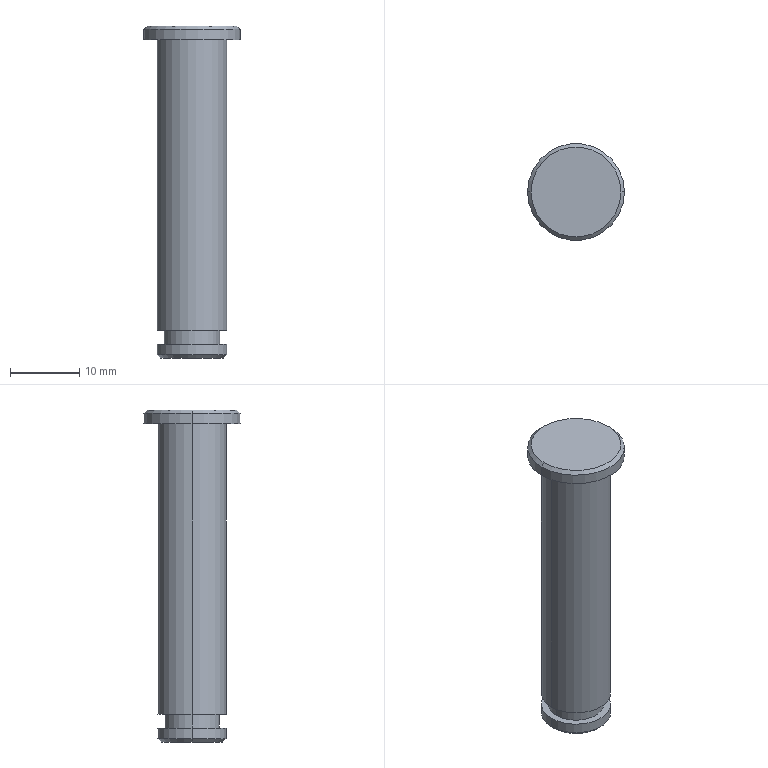Part | SolidWorks | features Chamfer 1, CutThin 1, Extrusion 1, ICE 1 | 1 solid | 17 faces | box 14 x 14 x 48 mm | volume 3855 mm3 | cylinder 8 | plane 5 | cone 4 | commonest cylinder face diameters 10 x4 8 x2 14 x2
STEP:
#1=CARTESIAN_POINT('',(-5.,0.,2.));
#2=VERTEX_POINT('',#1);
#3=CARTESIAN_POINT('',(5.,0.,2.));
#4=VERTEX_POINT('',#3);
#5=CARTESIAN_POINT('',(0.,0.,2.));
#6=DIRECTION('',(0.,0.,-1.));
#7=DIRECTION('',(-1.,0.,0.));
#8=AXIS2_PLACEMENT_3D('',#5,#6,#7);
#9=CIRCLE('',#8,5.);
#10=EDGE_CURVE('',#2,#4,#9,.T.);
#11=ORIENTED_EDGE('',*,*,#10,.T.);
#12=CARTESIAN_POINT('',(5.,0.,0.5));
#13=VERTEX_POINT('',#12);
#14=CARTESIAN_POINT('',(5.,0.,46.));
#15=DIRECTION('',(0.,0.,-1.));
#16=VECTOR('',#15,1000.);
#17=LINE('',#14,#16);
#18=EDGE_CURVE('',#4,#13,#17,.T.);
#19=ORIENTED_EDGE('',*,*,#18,.T.);
#20=CARTESIAN_POINT('',(-5.,0.,0.5));
#21=VERTEX_POINT('',#20);
#22=CARTESIAN_POINT('',(0.,0.,0.5));
#23=DIRECTION('',(0.,0.,1.));
#24=DIRECTION('',(1.,0.,0.));
#25=AXIS2_PLACEMENT_3D('',#22,#23,#24);
#26=CIRCLE('',#25,5.);
#27=EDGE_CURVE('',#13,#21,#26,.T.);
#28=ORIENTED_EDGE('',*,*,#27,.T.);
#29=CARTESIAN_POINT('',(-5.,0.,46.));
#30=DIRECTION('',(0.,0.,-1.));
#31=VECTOR('',#30,1000.);
#32=LINE('',#29,#31);
#33=EDGE_CURVE('',#2,#21,#32,.T.);
#34=ORIENTED_EDGE('',*,*,#33,.F.);
#35=EDGE_LOOP('',(#11,#19,#28,#34));
#36=FACE_OUTER_BOUND('',#35,.T.);
#37=CARTESIAN_POINT('',(0.,0.,46.));
#38=DIRECTION('',(0.,0.,-1.));
#39=DIRECTION('',(-1.,0.,0.));
#40=AXIS2_PLACEMENT_3D('',#37,#38,#39);
#41=CYLINDRICAL_SURFACE('',#40,5.);
#42=ADVANCED_FACE('',(#36),#41,.T.);
#43=CARTESIAN_POINT('',(-4.5,0.,0.));
#44=VERTEX_POINT('',#43);
#45=CARTESIAN_POINT('',(4.5,0.,0.));
#46=VERTEX_POINT('',#45);
#47=CARTESIAN_POINT('',(0.,0.,0.));
#48=DIRECTION('',(0.,0.,-1.));
#49=DIRECTION('',(1.,0.,0.));
#50=AXIS2_PLACEMENT_3D('',#47,#48,#49);
#51=CIRCLE('',#50,4.5);
#52=EDGE_CURVE('',#44,#46,#51,.T.);
#53=ORIENTED_EDGE('',*,*,#52,.F.);
#54=CARTESIAN_POINT('',(-5.,0.,0.5));
#55=DIRECTION('',(-0.7071,0.,0.7071));
#56=VECTOR('',#55,1000.);
#57=LINE('',#54,#56);
#58=EDGE_CURVE('',#44,#21,#57,.T.);
#59=ORIENTED_EDGE('',*,*,#58,.T.);
#60=ORIENTED_EDGE('',*,*,#27,.F.);
#61=CARTESIAN_POINT('',(5.,0.,0.5));
#62=DIRECTION('',(0.7071,0.,0.7071));
#63=VECTOR('',#62,1000.);
#64=LINE('',#61,#63);
#65=EDGE_CURVE('',#46,#13,#64,.T.);
#66=ORIENTED_EDGE('',*,*,#65,.F.);
#67=EDGE_LOOP('',(#53,#59,#60,#66));
#68=FACE_OUTER_BOUND('',#67,.T.);
#69=CARTESIAN_POINT('',(0.,0.,0.5));
#70=DIRECTION('',(0.,0.,1.));
#71=DIRECTION('',(1.,0.,0.));
#72=AXIS2_PLACEMENT_3D('',#69,#70,#71);
#73=CONICAL_SURFACE('',#72,5.,0.7854);
#74=ADVANCED_FACE('',(#68),#73,.T.);
#75=CARTESIAN_POINT('',(-4.,0.,4.));
#76=VERTEX_POINT('',#75);
#77=CARTESIAN_POINT('',(4.,0.,4.));
#78=VERTEX_POINT('',#77);
#79=CARTESIAN_POINT('',(0.,0.,4.));
#80=DIRECTION('',(0.,0.,-1.));
#81=DIRECTION('',(-1.,0.,0.));
#82=AXIS2_PLACEMENT_3D('',#79,#80,#81);
#83=CIRCLE('',#82,4.);
#84=EDGE_CURVE('',#76,#78,#83,.T.);
#85=ORIENTED_EDGE('',*,*,#84,.T.);
#86=CARTESIAN_POINT('',(4.,0.,2.));
#87=VERTEX_POINT('',#86);
#88=CARTESIAN_POINT('',(4.,0.,4.));
#89=DIRECTION('',(0.,0.,-1.));
#90=VECTOR('',#89,1000.);
#91=LINE('',#88,#90);
#92=EDGE_CURVE('',#78,#87,#91,.T.);
#93=ORIENTED_EDGE('',*,*,#92,.T.);
#94=CARTESIAN_POINT('',(-4.,0.,2.));
#95=VERTEX_POINT('',#94);
#96=CARTESIAN_POINT('',(0.,0.,2.));
#97=DIRECTION('',(0.,0.,-1.));
#98=DIRECTION('',(-1.,0.,0.));
#99=AXIS2_PLACEMENT_3D('',#96,#97,#98);
#100=CIRCLE('',#99,4.);
#101=EDGE_CURVE('',#95,#87,#100,.T.);
#102=ORIENTED_EDGE('',*,*,#101,.F.);
#103=CARTESIAN_POINT('',(-4.,0.,4.));
#104=DIRECTION('',(0.,0.,-1.));
#105=VECTOR('',#104,1000.);
#106=LINE('',#103,#105);
#107=EDGE_CURVE('',#76,#95,#106,.T.);
#108=ORIENTED_EDGE('',*,*,#107,.F.);
#109=EDGE_LOOP('',(#85,#93,#102,#108));
#110=FACE_OUTER_BOUND('',#109,.T.);
#111=CARTESIAN_POINT('',(0.,0.,4.));
#112=DIRECTION('',(0.,0.,-1.));
#113=DIRECTION('',(-1.,0.,0.));
#114=AXIS2_PLACEMENT_3D('',#111,#112,#113);
#115=CYLINDRICAL_SURFACE('',#114,4.);
#116=ADVANCED_FACE('',(#110),#115,.T.);
#117=CARTESIAN_POINT('',(6.5,0.,48.));
#118=VERTEX_POINT('',#117);
#119=CARTESIAN_POINT('',(-6.5,0.,48.));
#120=VERTEX_POINT('',#119);
#121=CARTESIAN_POINT('',(0.,0.,48.));
#122=DIRECTION('',(0.,0.,1.));
#123=DIRECTION('',(1.,0.,0.));
#124=AXIS2_PLACEMENT_3D('',#121,#122,#123);
#125=CIRCLE('',#124,6.5);
#126=EDGE_CURVE('',#118,#120,#125,.T.);
#127=ORIENTED_EDGE('',*,*,#126,.F.);
#128=CARTESIAN_POINT('',(7.,0.,47.5));
#129=VERTEX_POINT('',#128);
#130=CARTESIAN_POINT('',(6.5,0.,48.));
#131=DIRECTION('',(0.7071,0.,-0.7071));
#132=VECTOR('',#131,1000.);
#133=LINE('',#130,#132);
#134=EDGE_CURVE('',#118,#129,#133,.T.);
#135=ORIENTED_EDGE('',*,*,#134,.T.);
#136=CARTESIAN_POINT('',(-7.,0.,47.5));
#137=VERTEX_POINT('',#136);
#138=CARTESIAN_POINT('',(0.,0.,47.5));
#139=DIRECTION('',(0.,0.,-1.));
#140=DIRECTION('',(1.,0.,0.));
#141=AXIS2_PLACEMENT_3D('',#138,#139,#140);
#142=CIRCLE('',#141,7.);
#143=EDGE_CURVE('',#137,#129,#142,.T.);
#144=ORIENTED_EDGE('',*,*,#143,.F.);
#145=CARTESIAN_POINT('',(-6.5,0.,48.));
#146=DIRECTION('',(-0.7071,0.,-0.7071));
#147=VECTOR('',#146,1000.);
#148=LINE('',#145,#147);
#149=EDGE_CURVE('',#120,#137,#148,.T.);
#150=ORIENTED_EDGE('',*,*,#149,.F.);
#151=EDGE_LOOP('',(#127,#135,#144,#150));
#152=FACE_OUTER_BOUND('',#151,.T.);
#153=CARTESIAN_POINT('',(0.,0.,48.));
#154=DIRECTION('',(0.,0.,-1.));
#155=DIRECTION('',(-1.,0.,0.));
#156=AXIS2_PLACEMENT_3D('',#153,#154,#155);
#157=CONICAL_SURFACE('',#156,6.5,0.7854);
#158=ADVANCED_FACE('',(#152),#157,.T.);
#159=ORIENTED_EDGE('',*,*,#143,.T.);
#160=CARTESIAN_POINT('',(7.,0.,46.));
#161=VERTEX_POINT('',#160);
#162=CARTESIAN_POINT('',(7.,0.,48.));
#163=DIRECTION('',(0.,0.,-1.));
#164=VECTOR('',#163,1000.);
#165=LINE('',#162,#164);
#166=EDGE_CURVE('',#129,#161,#165,.T.);
#167=ORIENTED_EDGE('',*,*,#166,.T.);
#168=CARTESIAN_POINT('',(-7.,0.,46.));
#169=VERTEX_POINT('',#168);
#170=CARTESIAN_POINT('',(0.,0.,46.));
#171=DIRECTION('',(0.,0.,1.));
#172=DIRECTION('',(1.,0.,0.));
#173=AXIS2_PLACEMENT_3D('',#170,#171,#172);
#174=CIRCLE('',#173,7.);
#175=EDGE_CURVE('',#161,#169,#174,.T.);
#176=ORIENTED_EDGE('',*,*,#175,.T.);
#177=CARTESIAN_POINT('',(-7.,0.,48.));
#178=DIRECTION('',(0.,0.,-1.));
#179=VECTOR('',#178,1000.);
#180=LINE('',#177,#179);
#181=EDGE_CURVE('',#137,#169,#180,.T.);
#182=ORIENTED_EDGE('',*,*,#181,.F.);
#183=EDGE_LOOP('',(#159,#167,#176,#182));
#184=FACE_OUTER_BOUND('',#183,.T.);
#185=CARTESIAN_POINT('',(0.,0.,48.));
#186=DIRECTION('',(0.,0.,-1.));
#187=DIRECTION('',(-1.,0.,0.));
#188=AXIS2_PLACEMENT_3D('',#185,#186,#187);
#189=CYLINDRICAL_SURFACE('',#188,7.);
#190=ADVANCED_FACE('',(#184),#189,.T.);
#191=CARTESIAN_POINT('',(5.,0.,46.));
#192=VERTEX_POINT('',#191);
#193=CARTESIAN_POINT('',(-5.,0.,46.));
#194=VERTEX_POINT('',#193);
#195=CARTESIAN_POINT('',(0.,0.,46.));
#196=DIRECTION('',(0.,0.,1.));
#197=DIRECTION('',(1.,0.,0.));
#198=AXIS2_PLACEMENT_3D('',#195,#196,#197);
#199=CIRCLE('',#198,5.);
#200=EDGE_CURVE('',#192,#194,#199,.T.);
#201=ORIENTED_EDGE('',*,*,#200,.F.);
#202=CARTESIAN_POINT('',(5.,0.,4.));
#203=VERTEX_POINT('',#202);
#204=CARTESIAN_POINT('',(5.,0.,46.));
#205=DIRECTION('',(0.,0.,-1.));
#206=VECTOR('',#205,1000.);
#207=LINE('',#204,#206);
#208=EDGE_CURVE('',#192,#203,#207,.T.);
#209=ORIENTED_EDGE('',*,*,#208,.T.);
#210=CARTESIAN_POINT('',(-5.,0.,4.));
#211=VERTEX_POINT('',#210);
#212=CARTESIAN_POINT('',(0.,0.,4.));
#213=DIRECTION('',(0.,0.,-1.));
#214=DIRECTION('',(-1.,0.,0.));
#215=AXIS2_PLACEMENT_3D('',#212,#213,#214);
#216=CIRCLE('',#215,5.);
#217=EDGE_CURVE('',#211,#203,#216,.T.);
#218=ORIENTED_EDGE('',*,*,#217,.F.);
#219=CARTESIAN_POINT('',(-5.,0.,46.));
#220=DIRECTION('',(0.,0.,-1.));
#221=VECTOR('',#220,1000.);
#222=LINE('',#219,#221);
#223=EDGE_CURVE('',#194,#211,#222,.T.);
#224=ORIENTED_EDGE('',*,*,#223,.F.);
#225=EDGE_LOOP('',(#201,#209,#218,#224));
#226=FACE_OUTER_BOUND('',#225,.T.);
#227=CARTESIAN_POINT('',(0.,0.,46.));
#228=DIRECTION('',(0.,0.,-1.));
#229=DIRECTION('',(-1.,0.,0.));
#230=AXIS2_PLACEMENT_3D('',#227,#228,#229);
#231=CYLINDRICAL_SURFACE('',#230,5.);
#232=ADVANCED_FACE('',(#226),#231,.T.);
#233=ORIENTED_EDGE('',*,*,#208,.F.);
#234=CARTESIAN_POINT('',(0.,0.,46.));
#235=DIRECTION('',(0.,0.,1.));
#236=DIRECTION('',(1.,0.,0.));
#237=AXIS2_PLACEMENT_3D('',#234,#235,#236);
#238=CIRCLE('',#237,5.);
#239=EDGE_CURVE('',#194,#192,#238,.T.);
#240=ORIENTED_EDGE('',*,*,#239,.F.);
#241=ORIENTED_EDGE('',*,*,#223,.T.);
#242=CARTESIAN_POINT('',(0.,0.,4.));
#243=DIRECTION('',(0.,0.,-1.));
#244=DIRECTION('',(-1.,0.,0.));
#245=AXIS2_PLACEMENT_3D('',#242,#243,#244);
#246=CIRCLE('',#245,5.);
#247=EDGE_CURVE('',#203,#211,#246,.T.);
#248=ORIENTED_EDGE('',*,*,#247,.F.);
#249=EDGE_LOOP('',(#233,#240,#241,#248));
#250=FACE_OUTER_BOUND('',#249,.T.);
#251=CARTESIAN_POINT('',(0.,0.,46.));
#252=DIRECTION('',(0.,0.,-1.));
#253=DIRECTION('',(-1.,0.,0.));
#254=AXIS2_PLACEMENT_3D('',#251,#252,#253);
#255=CYLINDRICAL_SURFACE('',#254,5.);
#256=ADVANCED_FACE('',(#250),#255,.T.);
#257=ORIENTED_EDGE('',*,*,#166,.F.);
#258=CARTESIAN_POINT('',(0.,0.,47.5));
#259=DIRECTION('',(0.,0.,-1.));
#260=DIRECTION('',(1.,0.,0.));
#261=AXIS2_PLACEMENT_3D('',#258,#259,#260);
#262=CIRCLE('',#261,7.);
#263=EDGE_CURVE('',#129,#137,#262,.T.);
#264=ORIENTED_EDGE('',*,*,#263,.T.);
#265=ORIENTED_EDGE('',*,*,#181,.T.);
#266=CARTESIAN_POINT('',(0.,0.,46.));
#267=DIRECTION('',(0.,0.,1.));
#268=DIRECTION('',(1.,0.,0.));
#269=AXIS2_PLACEMENT_3D('',#266,#267,#268);
#270=CIRCLE('',#269,7.);
#271=EDGE_CURVE('',#169,#161,#270,.T.);
#272=ORIENTED_EDGE('',*,*,#271,.T.);
#273=EDGE_LOOP('',(#257,#264,#265,#272));
#274=FACE_OUTER_BOUND('',#273,.T.);
#275=CARTESIAN_POINT('',(0.,0.,48.));
#276=DIRECTION('',(0.,0.,-1.));
#277=DIRECTION('',(-1.,0.,0.));
#278=AXIS2_PLACEMENT_3D('',#275,#276,#277);
#279=CYLINDRICAL_SURFACE('',#278,7.);
#280=ADVANCED_FACE('',(#274),#279,.T.);
#281=CARTESIAN_POINT('',(0.,0.,48.));
#282=DIRECTION('',(0.,0.,1.));
#283=DIRECTION('',(1.,0.,0.));
#284=AXIS2_PLACEMENT_3D('',#281,#282,#283);
#285=CIRCLE('',#284,6.5);
#286=EDGE_CURVE('',#120,#118,#285,.T.);
#287=ORIENTED_EDGE('',*,*,#286,.T.);
#288=ORIENTED_EDGE('',*,*,#126,.T.);
#289=EDGE_LOOP('',(#287,#288));
#290=FACE_OUTER_BOUND('',#289,.T.);
#291=CARTESIAN_POINT('',(0.,0.,48.));
#292=DIRECTION('',(0.,0.,1.));
#293=DIRECTION('',(1.,0.,0.));
#294=AXIS2_PLACEMENT_3D('',#291,#292,#293);
#295=PLANE('',#294);
#296=ADVANCED_FACE('',(#290),#295,.T.);
#297=ORIENTED_EDGE('',*,*,#239,.T.);
#298=ORIENTED_EDGE('',*,*,#200,.T.);
#299=EDGE_LOOP('',(#297,#298));
#300=FACE_BOUND('',#299,.T.);
#301=ORIENTED_EDGE('',*,*,#271,.F.);
#302=ORIENTED_EDGE('',*,*,#175,.F.);
#303=EDGE_LOOP('',(#301,#302));
#304=FACE_OUTER_BOUND('',#303,.T.);
#305=CARTESIAN_POINT('',(0.,0.,46.));
#306=DIRECTION('',(0.,0.,1.));
#307=DIRECTION('',(1.,0.,0.));
#308=AXIS2_PLACEMENT_3D('',#305,#306,#307);
#309=PLANE('',#308);
#310=ADVANCED_FACE('',(#300,#304),#309,.F.);
#311=ORIENTED_EDGE('',*,*,#134,.F.);
#312=ORIENTED_EDGE('',*,*,#286,.F.);
#313=ORIENTED_EDGE('',*,*,#149,.T.);
#314=ORIENTED_EDGE('',*,*,#263,.F.);
#315=EDGE_LOOP('',(#311,#312,#313,#314));
#316=FACE_OUTER_BOUND('',#315,.T.);
#317=CARTESIAN_POINT('',(0.,0.,48.));
#318=DIRECTION('',(0.,0.,-1.));
#319=DIRECTION('',(-1.,0.,0.));
#320=AXIS2_PLACEMENT_3D('',#317,#318,#319);
#321=CONICAL_SURFACE('',#320,6.5,0.7854);
#322=ADVANCED_FACE('',(#316),#321,.T.);
#323=ORIENTED_EDGE('',*,*,#84,.F.);
#324=CARTESIAN_POINT('',(0.,0.,4.));
#325=DIRECTION('',(0.,0.,-1.));
#326=DIRECTION('',(-1.,0.,0.));
#327=AXIS2_PLACEMENT_3D('',#324,#325,#326);
#328=CIRCLE('',#327,4.);
#329=EDGE_CURVE('',#78,#76,#328,.T.);
#330=ORIENTED_EDGE('',*,*,#329,.F.);
#331=EDGE_LOOP('',(#323,#330));
#332=FACE_BOUND('',#331,.T.);
#333=ORIENTED_EDGE('',*,*,#217,.T.);
#334=ORIENTED_EDGE('',*,*,#247,.T.);
#335=EDGE_LOOP('',(#333,#334));
#336=FACE_OUTER_BOUND('',#335,.T.);
#337=CARTESIAN_POINT('',(0.,0.,4.));
#338=DIRECTION('',(0.,0.,-1.));
#339=DIRECTION('',(-1.,0.,0.));
#340=AXIS2_PLACEMENT_3D('',#337,#338,#339);
#341=PLANE('',#340);
#342=ADVANCED_FACE('',(#332,#336),#341,.T.);
#343=ORIENTED_EDGE('',*,*,#101,.T.);
#344=CARTESIAN_POINT('',(0.,0.,2.));
#345=DIRECTION('',(0.,0.,-1.));
#346=DIRECTION('',(-1.,0.,0.));
#347=AXIS2_PLACEMENT_3D('',#344,#345,#346);
#348=CIRCLE('',#347,4.);
#349=EDGE_CURVE('',#87,#95,#348,.T.);
#350=ORIENTED_EDGE('',*,*,#349,.T.);
#351=EDGE_LOOP('',(#343,#350));
#352=FACE_BOUND('',#351,.T.);
#353=ORIENTED_EDGE('',*,*,#10,.F.);
#354=CARTESIAN_POINT('',(0.,0.,2.));
#355=DIRECTION('',(0.,0.,-1.));
#356=DIRECTION('',(-1.,0.,0.));
#357=AXIS2_PLACEMENT_3D('',#354,#355,#356);
#358=CIRCLE('',#357,5.);
#359=EDGE_CURVE('',#4,#2,#358,.T.);
#360=ORIENTED_EDGE('',*,*,#359,.F.);
#361=EDGE_LOOP('',(#353,#360));
#362=FACE_OUTER_BOUND('',#361,.T.);
#363=CARTESIAN_POINT('',(0.,0.,2.));
#364=DIRECTION('',(0.,0.,-1.));
#365=DIRECTION('',(-1.,0.,0.));
#366=AXIS2_PLACEMENT_3D('',#363,#364,#365);
#367=PLANE('',#366);
#368=ADVANCED_FACE('',(#352,#362),#367,.F.);
#369=ORIENTED_EDGE('',*,*,#92,.F.);
#370=ORIENTED_EDGE('',*,*,#329,.T.);
#371=ORIENTED_EDGE('',*,*,#107,.T.);
#372=ORIENTED_EDGE('',*,*,#349,.F.);
#373=EDGE_LOOP('',(#369,#370,#371,#372));
#374=FACE_OUTER_BOUND('',#373,.T.);
#375=CARTESIAN_POINT('',(0.,0.,4.));
#376=DIRECTION('',(0.,0.,-1.));
#377=DIRECTION('',(-1.,0.,0.));
#378=AXIS2_PLACEMENT_3D('',#375,#376,#377);
#379=CYLINDRICAL_SURFACE('',#378,4.);
#380=ADVANCED_FACE('',(#374),#379,.T.);
#381=CARTESIAN_POINT('',(0.,0.,0.));
#382=DIRECTION('',(0.,0.,-1.));
#383=DIRECTION('',(1.,0.,0.));
#384=AXIS2_PLACEMENT_3D('',#381,#382,#383);
#385=CIRCLE('',#384,4.5);
#386=EDGE_CURVE('',#46,#44,#385,.T.);
#387=ORIENTED_EDGE('',*,*,#386,.T.);
#388=ORIENTED_EDGE('',*,*,#52,.T.);
#389=EDGE_LOOP('',(#387,#388));
#390=FACE_OUTER_BOUND('',#389,.T.);
#391=CARTESIAN_POINT('',(0.,0.,0.));
#392=DIRECTION('',(0.,0.,1.));
#393=DIRECTION('',(1.,0.,0.));
#394=AXIS2_PLACEMENT_3D('',#391,#392,#393);
#395=PLANE('',#394);
#396=ADVANCED_FACE('',(#390),#395,.F.);
#397=ORIENTED_EDGE('',*,*,#58,.F.);
#398=ORIENTED_EDGE('',*,*,#386,.F.);
#399=ORIENTED_EDGE('',*,*,#65,.T.);
#400=CARTESIAN_POINT('',(0.,0.,0.5));
#401=DIRECTION('',(0.,0.,1.));
#402=DIRECTION('',(1.,0.,0.));
#403=AXIS2_PLACEMENT_3D('',#400,#401,#402);
#404=CIRCLE('',#403,5.);
#405=EDGE_CURVE('',#21,#13,#404,.T.);
#406=ORIENTED_EDGE('',*,*,#405,.F.);
#407=EDGE_LOOP('',(#397,#398,#399,#406));
#408=FACE_OUTER_BOUND('',#407,.T.);
#409=CARTESIAN_POINT('',(0.,0.,0.5));
#410=DIRECTION('',(0.,0.,1.));
#411=DIRECTION('',(1.,0.,0.));
#412=AXIS2_PLACEMENT_3D('',#409,#410,#411);
#413=CONICAL_SURFACE('',#412,5.,0.7854);
#414=ADVANCED_FACE('',(#408),#413,.T.);
#415=ORIENTED_EDGE('',*,*,#18,.F.);
#416=ORIENTED_EDGE('',*,*,#359,.T.);
#417=ORIENTED_EDGE('',*,*,#33,.T.);
#418=ORIENTED_EDGE('',*,*,#405,.T.);
#419=EDGE_LOOP('',(#415,#416,#417,#418));
#420=FACE_OUTER_BOUND('',#419,.T.);
#421=CARTESIAN_POINT('',(0.,0.,46.));
#422=DIRECTION('',(0.,0.,-1.));
#423=DIRECTION('',(-1.,0.,0.));
#424=AXIS2_PLACEMENT_3D('',#421,#422,#423);
#425=CYLINDRICAL_SURFACE('',#424,5.);
#426=ADVANCED_FACE('',(#420),#425,.T.);
#427=CLOSED_SHELL('',(#42,#74,#116,#158,#190,#232,#256,#280,#296,#310,#322,#342,#368,#380,#396,#414,#426));
#428=MANIFOLD_SOLID_BREP('',#427);
#429=CARTESIAN_POINT('',(0.,0.,0.));
#430=DIRECTION('',(0.,0.,1.));
#431=DIRECTION('',(1.,0.,0.));
#432=AXIS2_PLACEMENT_3D('',#429,#430,#431);
#433=(LENGTH_UNIT()NAMED_UNIT(*)SI_UNIT(.MILLI.,.METRE.));
#434=UNCERTAINTY_MEASURE_WITH_UNIT(LENGTH_MEASURE(0.00001),#433,'','');
#435=(NAMED_UNIT(*)PLANE_ANGLE_UNIT()SI_UNIT($,.RADIAN.));
#436=(NAMED_UNIT(*)SI_UNIT($,.STERADIAN.)SOLID_ANGLE_UNIT());
#437=(GEOMETRIC_REPRESENTATION_CONTEXT(3)GLOBAL_UNCERTAINTY_ASSIGNED_CONTEXT((#434))GLOBAL_UNIT_ASSIGNED_CONTEXT((#433,#435,#436))REPRESENTATION_CONTEXT('',''));
#438=ADVANCED_BREP_SHAPE_REPRESENTATION('',(#428,#432),#437);